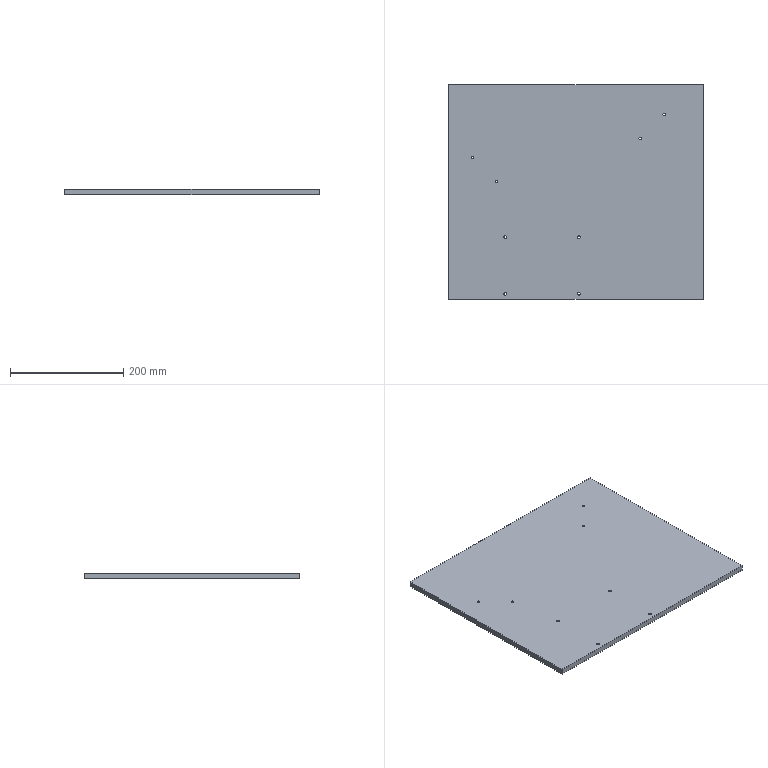Part | STEP file | 11-123211 | 1 solid | 22 faces | box 450 x 380 x 10 mm | volume 1708660 mm3 | cylinder 16 | plane 6 | commonest cylinder face diameters 4.2 x8 5 x8
STEP:
#1=CARTESIAN_POINT('',(153.683,136.933,10.));
#2=VERTEX_POINT('',#1);
#3=CARTESIAN_POINT('',(157.883,136.933,10.));
#4=VERTEX_POINT('',#3);
#5=CARTESIAN_POINT('',(155.783,136.933,10.));
#6=DIRECTION('',(0.,0.,1.));
#7=DIRECTION('',(1.,0.,0.));
#8=AXIS2_PLACEMENT_3D('',#5,#6,#7);
#9=CIRCLE('',#8,2.1);
#10=EDGE_CURVE('',#2,#4,#9,.T.);
#11=ORIENTED_EDGE('',*,*,#10,.T.);
#12=CARTESIAN_POINT('',(157.883,136.933,0.));
#13=VERTEX_POINT('',#12);
#14=CARTESIAN_POINT('',(157.883,136.933,0.));
#15=DIRECTION('',(0.,0.,-1.));
#16=VECTOR('',#15,1000.);
#17=LINE('',#14,#16);
#18=EDGE_CURVE('',#4,#13,#17,.T.);
#19=ORIENTED_EDGE('',*,*,#18,.T.);
#20=CARTESIAN_POINT('',(153.683,136.933,0.));
#21=VERTEX_POINT('',#20);
#22=CARTESIAN_POINT('',(155.783,136.933,0.));
#23=DIRECTION('',(0.,0.,-1.));
#24=DIRECTION('',(-1.,0.,0.));
#25=AXIS2_PLACEMENT_3D('',#22,#23,#24);
#26=CIRCLE('',#25,2.1);
#27=EDGE_CURVE('',#13,#21,#26,.T.);
#28=ORIENTED_EDGE('',*,*,#27,.T.);
#29=CARTESIAN_POINT('',(153.683,136.933,0.));
#30=DIRECTION('',(0.,0.,-1.));
#31=VECTOR('',#30,1000.);
#32=LINE('',#29,#31);
#33=EDGE_CURVE('',#2,#21,#32,.T.);
#34=ORIENTED_EDGE('',*,*,#33,.F.);
#35=EDGE_LOOP('',(#11,#19,#28,#34));
#36=FACE_OUTER_BOUND('',#35,.T.);
#37=CARTESIAN_POINT('',(155.783,136.933,0.));
#38=DIRECTION('',(0.,0.,-1.));
#39=DIRECTION('',(-1.,0.,0.));
#40=AXIS2_PLACEMENT_3D('',#37,#38,#39);
#41=CYLINDRICAL_SURFACE('',#40,2.1);
#42=ADVANCED_FACE('',(#36),#41,.F.);
#43=CARTESIAN_POINT('',(111.257,94.507,10.));
#44=VERTEX_POINT('',#43);
#45=CARTESIAN_POINT('',(115.457,94.507,10.));
#46=VERTEX_POINT('',#45);
#47=CARTESIAN_POINT('',(113.357,94.507,10.));
#48=DIRECTION('',(0.,0.,1.));
#49=DIRECTION('',(1.,0.,0.));
#50=AXIS2_PLACEMENT_3D('',#47,#48,#49);
#51=CIRCLE('',#50,2.1);
#52=EDGE_CURVE('',#44,#46,#51,.T.);
#53=ORIENTED_EDGE('',*,*,#52,.T.);
#54=CARTESIAN_POINT('',(115.457,94.507,0.));
#55=VERTEX_POINT('',#54);
#56=CARTESIAN_POINT('',(115.457,94.507,0.));
#57=DIRECTION('',(0.,0.,-1.));
#58=VECTOR('',#57,1000.);
#59=LINE('',#56,#58);
#60=EDGE_CURVE('',#46,#55,#59,.T.);
#61=ORIENTED_EDGE('',*,*,#60,.T.);
#62=CARTESIAN_POINT('',(111.257,94.507,0.));
#63=VERTEX_POINT('',#62);
#64=CARTESIAN_POINT('',(113.357,94.507,0.));
#65=DIRECTION('',(0.,0.,-1.));
#66=DIRECTION('',(-1.,0.,0.));
#67=AXIS2_PLACEMENT_3D('',#64,#65,#66);
#68=CIRCLE('',#67,2.1);
#69=EDGE_CURVE('',#55,#63,#68,.T.);
#70=ORIENTED_EDGE('',*,*,#69,.T.);
#71=CARTESIAN_POINT('',(111.257,94.507,0.));
#72=DIRECTION('',(0.,0.,-1.));
#73=VECTOR('',#72,1000.);
#74=LINE('',#71,#73);
#75=EDGE_CURVE('',#44,#63,#74,.T.);
#76=ORIENTED_EDGE('',*,*,#75,.F.);
#77=EDGE_LOOP('',(#53,#61,#70,#76));
#78=FACE_OUTER_BOUND('',#77,.T.);
#79=CARTESIAN_POINT('',(113.357,94.507,0.));
#80=DIRECTION('',(0.,0.,-1.));
#81=DIRECTION('',(-1.,0.,0.));
#82=AXIS2_PLACEMENT_3D('',#79,#80,#81);
#83=CYLINDRICAL_SURFACE('',#82,2.1);
#84=ADVANCED_FACE('',(#78),#83,.F.);
#85=CARTESIAN_POINT('',(-142.258,19.056,10.));
#86=VERTEX_POINT('',#85);
#87=CARTESIAN_POINT('',(-138.058,19.056,10.));
#88=VERTEX_POINT('',#87);
#89=CARTESIAN_POINT('',(-140.158,19.056,10.));
#90=DIRECTION('',(0.,0.,1.));
#91=DIRECTION('',(1.,0.,0.));
#92=AXIS2_PLACEMENT_3D('',#89,#90,#91);
#93=CIRCLE('',#92,2.1);
#94=EDGE_CURVE('',#86,#88,#93,.T.);
#95=ORIENTED_EDGE('',*,*,#94,.T.);
#96=CARTESIAN_POINT('',(-138.058,19.056,0.));
#97=VERTEX_POINT('',#96);
#98=CARTESIAN_POINT('',(-138.058,19.056,0.));
#99=DIRECTION('',(0.,0.,-1.));
#100=VECTOR('',#99,1000.);
#101=LINE('',#98,#100);
#102=EDGE_CURVE('',#88,#97,#101,.T.);
#103=ORIENTED_EDGE('',*,*,#102,.T.);
#104=CARTESIAN_POINT('',(-142.258,19.056,0.));
#105=VERTEX_POINT('',#104);
#106=CARTESIAN_POINT('',(-140.158,19.056,0.));
#107=DIRECTION('',(0.,0.,-1.));
#108=DIRECTION('',(-1.,0.,0.));
#109=AXIS2_PLACEMENT_3D('',#106,#107,#108);
#110=CIRCLE('',#109,2.1);
#111=EDGE_CURVE('',#97,#105,#110,.T.);
#112=ORIENTED_EDGE('',*,*,#111,.T.);
#113=CARTESIAN_POINT('',(-142.258,19.056,0.));
#114=DIRECTION('',(0.,0.,-1.));
#115=VECTOR('',#114,1000.);
#116=LINE('',#113,#115);
#117=EDGE_CURVE('',#86,#105,#116,.T.);
#118=ORIENTED_EDGE('',*,*,#117,.F.);
#119=EDGE_LOOP('',(#95,#103,#112,#118));
#120=FACE_OUTER_BOUND('',#119,.T.);
#121=CARTESIAN_POINT('',(-140.158,19.056,0.));
#122=DIRECTION('',(0.,0.,-1.));
#123=DIRECTION('',(-1.,0.,0.));
#124=AXIS2_PLACEMENT_3D('',#121,#122,#123);
#125=CYLINDRICAL_SURFACE('',#124,2.1);
#126=ADVANCED_FACE('',(#120),#125,.F.);
#127=CARTESIAN_POINT('',(-184.684,61.483,10.));
#128=VERTEX_POINT('',#127);
#129=CARTESIAN_POINT('',(-180.484,61.483,10.));
#130=VERTEX_POINT('',#129);
#131=CARTESIAN_POINT('',(-182.584,61.483,10.));
#132=DIRECTION('',(0.,0.,1.));
#133=DIRECTION('',(1.,0.,0.));
#134=AXIS2_PLACEMENT_3D('',#131,#132,#133);
#135=CIRCLE('',#134,2.1);
#136=EDGE_CURVE('',#128,#130,#135,.T.);
#137=ORIENTED_EDGE('',*,*,#136,.T.);
#138=CARTESIAN_POINT('',(-180.484,61.483,0.));
#139=VERTEX_POINT('',#138);
#140=CARTESIAN_POINT('',(-180.484,61.483,0.));
#141=DIRECTION('',(0.,0.,-1.));
#142=VECTOR('',#141,1000.);
#143=LINE('',#140,#142);
#144=EDGE_CURVE('',#130,#139,#143,.T.);
#145=ORIENTED_EDGE('',*,*,#144,.T.);
#146=CARTESIAN_POINT('',(-184.684,61.483,0.));
#147=VERTEX_POINT('',#146);
#148=CARTESIAN_POINT('',(-182.584,61.483,0.));
#149=DIRECTION('',(0.,0.,-1.));
#150=DIRECTION('',(-1.,0.,0.));
#151=AXIS2_PLACEMENT_3D('',#148,#149,#150);
#152=CIRCLE('',#151,2.1);
#153=EDGE_CURVE('',#139,#147,#152,.T.);
#154=ORIENTED_EDGE('',*,*,#153,.T.);
#155=CARTESIAN_POINT('',(-184.684,61.483,0.));
#156=DIRECTION('',(0.,0.,-1.));
#157=VECTOR('',#156,1000.);
#158=LINE('',#155,#157);
#159=EDGE_CURVE('',#128,#147,#158,.T.);
#160=ORIENTED_EDGE('',*,*,#159,.F.);
#161=EDGE_LOOP('',(#137,#145,#154,#160));
#162=FACE_OUTER_BOUND('',#161,.T.);
#163=CARTESIAN_POINT('',(-182.584,61.483,0.));
#164=DIRECTION('',(0.,0.,-1.));
#165=DIRECTION('',(-1.,0.,0.));
#166=AXIS2_PLACEMENT_3D('',#163,#164,#165);
#167=CYLINDRICAL_SURFACE('',#166,2.1);
#168=ADVANCED_FACE('',(#162),#167,.F.);
#169=CARTESIAN_POINT('',(-127.5,-80.,10.));
#170=VERTEX_POINT('',#169);
#171=CARTESIAN_POINT('',(-122.5,-80.,10.));
#172=VERTEX_POINT('',#171);
#173=CARTESIAN_POINT('',(-125.,-80.,10.));
#174=DIRECTION('',(0.,0.,1.));
#175=DIRECTION('',(1.,0.,0.));
#176=AXIS2_PLACEMENT_3D('',#173,#174,#175);
#177=CIRCLE('',#176,2.5);
#178=EDGE_CURVE('',#170,#172,#177,.T.);
#179=ORIENTED_EDGE('',*,*,#178,.T.);
#180=CARTESIAN_POINT('',(-122.5,-80.,0.));
#181=VERTEX_POINT('',#180);
#182=CARTESIAN_POINT('',(-122.5,-80.,0.));
#183=DIRECTION('',(0.,0.,-1.));
#184=VECTOR('',#183,1000.);
#185=LINE('',#182,#184);
#186=EDGE_CURVE('',#172,#181,#185,.T.);
#187=ORIENTED_EDGE('',*,*,#186,.T.);
#188=CARTESIAN_POINT('',(-127.5,-80.,0.));
#189=VERTEX_POINT('',#188);
#190=CARTESIAN_POINT('',(-125.,-80.,0.));
#191=DIRECTION('',(0.,0.,-1.));
#192=DIRECTION('',(-1.,0.,0.));
#193=AXIS2_PLACEMENT_3D('',#190,#191,#192);
#194=CIRCLE('',#193,2.5);
#195=EDGE_CURVE('',#181,#189,#194,.T.);
#196=ORIENTED_EDGE('',*,*,#195,.T.);
#197=CARTESIAN_POINT('',(-127.5,-80.,0.));
#198=DIRECTION('',(0.,0.,-1.));
#199=VECTOR('',#198,1000.);
#200=LINE('',#197,#199);
#201=EDGE_CURVE('',#170,#189,#200,.T.);
#202=ORIENTED_EDGE('',*,*,#201,.F.);
#203=EDGE_LOOP('',(#179,#187,#196,#202));
#204=FACE_OUTER_BOUND('',#203,.T.);
#205=CARTESIAN_POINT('',(-125.,-80.,0.));
#206=DIRECTION('',(0.,0.,-1.));
#207=DIRECTION('',(-1.,0.,0.));
#208=AXIS2_PLACEMENT_3D('',#205,#206,#207);
#209=CYLINDRICAL_SURFACE('',#208,2.5);
#210=ADVANCED_FACE('',(#204),#209,.F.);
#211=CARTESIAN_POINT('',(-127.5,-180.,10.));
#212=VERTEX_POINT('',#211);
#213=CARTESIAN_POINT('',(-122.5,-180.,10.));
#214=VERTEX_POINT('',#213);
#215=CARTESIAN_POINT('',(-125.,-180.,10.));
#216=DIRECTION('',(0.,0.,1.));
#217=DIRECTION('',(1.,0.,0.));
#218=AXIS2_PLACEMENT_3D('',#215,#216,#217);
#219=CIRCLE('',#218,2.5);
#220=EDGE_CURVE('',#212,#214,#219,.T.);
#221=ORIENTED_EDGE('',*,*,#220,.T.);
#222=CARTESIAN_POINT('',(-122.5,-180.,0.));
#223=VERTEX_POINT('',#222);
#224=CARTESIAN_POINT('',(-122.5,-180.,0.));
#225=DIRECTION('',(0.,0.,-1.));
#226=VECTOR('',#225,1000.);
#227=LINE('',#224,#226);
#228=EDGE_CURVE('',#214,#223,#227,.T.);
#229=ORIENTED_EDGE('',*,*,#228,.T.);
#230=CARTESIAN_POINT('',(-127.5,-180.,0.));
#231=VERTEX_POINT('',#230);
#232=CARTESIAN_POINT('',(-125.,-180.,0.));
#233=DIRECTION('',(0.,0.,-1.));
#234=DIRECTION('',(-1.,0.,0.));
#235=AXIS2_PLACEMENT_3D('',#232,#233,#234);
#236=CIRCLE('',#235,2.5);
#237=EDGE_CURVE('',#223,#231,#236,.T.);
#238=ORIENTED_EDGE('',*,*,#237,.T.);
#239=CARTESIAN_POINT('',(-127.5,-180.,0.));
#240=DIRECTION('',(0.,0.,-1.));
#241=VECTOR('',#240,1000.);
#242=LINE('',#239,#241);
#243=EDGE_CURVE('',#212,#231,#242,.T.);
#244=ORIENTED_EDGE('',*,*,#243,.F.);
#245=EDGE_LOOP('',(#221,#229,#238,#244));
#246=FACE_OUTER_BOUND('',#245,.T.);
#247=CARTESIAN_POINT('',(-125.,-180.,0.));
#248=DIRECTION('',(0.,0.,-1.));
#249=DIRECTION('',(-1.,0.,0.));
#250=AXIS2_PLACEMENT_3D('',#247,#248,#249);
#251=CYLINDRICAL_SURFACE('',#250,2.5);
#252=ADVANCED_FACE('',(#246),#251,.F.);
#253=CARTESIAN_POINT('',(2.5,-180.,10.));
#254=VERTEX_POINT('',#253);
#255=CARTESIAN_POINT('',(7.5,-180.,10.));
#256=VERTEX_POINT('',#255);
#257=CARTESIAN_POINT('',(5.,-180.,10.));
#258=DIRECTION('',(0.,0.,1.));
#259=DIRECTION('',(1.,0.,0.));
#260=AXIS2_PLACEMENT_3D('',#257,#258,#259);
#261=CIRCLE('',#260,2.5);
#262=EDGE_CURVE('',#254,#256,#261,.T.);
#263=ORIENTED_EDGE('',*,*,#262,.T.);
#264=CARTESIAN_POINT('',(7.5,-180.,0.));
#265=VERTEX_POINT('',#264);
#266=CARTESIAN_POINT('',(7.5,-180.,0.));
#267=DIRECTION('',(0.,0.,-1.));
#268=VECTOR('',#267,1000.);
#269=LINE('',#266,#268);
#270=EDGE_CURVE('',#256,#265,#269,.T.);
#271=ORIENTED_EDGE('',*,*,#270,.T.);
#272=CARTESIAN_POINT('',(2.5,-180.,0.));
#273=VERTEX_POINT('',#272);
#274=CARTESIAN_POINT('',(5.,-180.,0.));
#275=DIRECTION('',(0.,0.,-1.));
#276=DIRECTION('',(-1.,0.,0.));
#277=AXIS2_PLACEMENT_3D('',#274,#275,#276);
#278=CIRCLE('',#277,2.5);
#279=EDGE_CURVE('',#265,#273,#278,.T.);
#280=ORIENTED_EDGE('',*,*,#279,.T.);
#281=CARTESIAN_POINT('',(2.5,-180.,0.));
#282=DIRECTION('',(0.,0.,-1.));
#283=VECTOR('',#282,1000.);
#284=LINE('',#281,#283);
#285=EDGE_CURVE('',#254,#273,#284,.T.);
#286=ORIENTED_EDGE('',*,*,#285,.F.);
#287=EDGE_LOOP('',(#263,#271,#280,#286));
#288=FACE_OUTER_BOUND('',#287,.T.);
#289=CARTESIAN_POINT('',(5.,-180.,0.));
#290=DIRECTION('',(0.,0.,-1.));
#291=DIRECTION('',(-1.,0.,0.));
#292=AXIS2_PLACEMENT_3D('',#289,#290,#291);
#293=CYLINDRICAL_SURFACE('',#292,2.5);
#294=ADVANCED_FACE('',(#288),#293,.F.);
#295=CARTESIAN_POINT('',(2.5,-80.,10.));
#296=VERTEX_POINT('',#295);
#297=CARTESIAN_POINT('',(7.5,-80.,10.));
#298=VERTEX_POINT('',#297);
#299=CARTESIAN_POINT('',(5.,-80.,10.));
#300=DIRECTION('',(0.,0.,1.));
#301=DIRECTION('',(1.,0.,0.));
#302=AXIS2_PLACEMENT_3D('',#299,#300,#301);
#303=CIRCLE('',#302,2.5);
#304=EDGE_CURVE('',#296,#298,#303,.T.);
#305=ORIENTED_EDGE('',*,*,#304,.T.);
#306=CARTESIAN_POINT('',(7.5,-80.,0.));
#307=VERTEX_POINT('',#306);
#308=CARTESIAN_POINT('',(7.5,-80.,0.));
#309=DIRECTION('',(0.,0.,-1.));
#310=VECTOR('',#309,1000.);
#311=LINE('',#308,#310);
#312=EDGE_CURVE('',#298,#307,#311,.T.);
#313=ORIENTED_EDGE('',*,*,#312,.T.);
#314=CARTESIAN_POINT('',(2.5,-80.,0.));
#315=VERTEX_POINT('',#314);
#316=CARTESIAN_POINT('',(5.,-80.,0.));
#317=DIRECTION('',(0.,0.,-1.));
#318=DIRECTION('',(-1.,0.,0.));
#319=AXIS2_PLACEMENT_3D('',#316,#317,#318);
#320=CIRCLE('',#319,2.5);
#321=EDGE_CURVE('',#307,#315,#320,.T.);
#322=ORIENTED_EDGE('',*,*,#321,.T.);
#323=CARTESIAN_POINT('',(2.5,-80.,0.));
#324=DIRECTION('',(0.,0.,-1.));
#325=VECTOR('',#324,1000.);
#326=LINE('',#323,#325);
#327=EDGE_CURVE('',#296,#315,#326,.T.);
#328=ORIENTED_EDGE('',*,*,#327,.F.);
#329=EDGE_LOOP('',(#305,#313,#322,#328));
#330=FACE_OUTER_BOUND('',#329,.T.);
#331=CARTESIAN_POINT('',(5.,-80.,0.));
#332=DIRECTION('',(0.,0.,-1.));
#333=DIRECTION('',(-1.,0.,0.));
#334=AXIS2_PLACEMENT_3D('',#331,#332,#333);
#335=CYLINDRICAL_SURFACE('',#334,2.5);
#336=ADVANCED_FACE('',(#330),#335,.F.);
#337=CARTESIAN_POINT('',(225.,-190.,0.));
#338=VERTEX_POINT('',#337);
#339=CARTESIAN_POINT('',(225.,190.,0.));
#340=VERTEX_POINT('',#339);
#341=CARTESIAN_POINT('',(225.,190.,0.));
#342=DIRECTION('',(0.,1.,0.));
#343=VECTOR('',#342,1000.);
#344=LINE('',#341,#343);
#345=EDGE_CURVE('',#338,#340,#344,.T.);
#346=ORIENTED_EDGE('',*,*,#345,.T.);
#347=CARTESIAN_POINT('',(225.,190.,10.));
#348=VERTEX_POINT('',#347);
#349=CARTESIAN_POINT('',(225.,190.,10.));
#350=DIRECTION('',(0.,0.,-1.));
#351=VECTOR('',#350,1000.);
#352=LINE('',#349,#351);
#353=EDGE_CURVE('',#348,#340,#352,.T.);
#354=ORIENTED_EDGE('',*,*,#353,.F.);
#355=CARTESIAN_POINT('',(225.,-190.,10.));
#356=VERTEX_POINT('',#355);
#357=CARTESIAN_POINT('',(225.,190.,10.));
#358=DIRECTION('',(0.,1.,0.));
#359=VECTOR('',#358,1000.);
#360=LINE('',#357,#359);
#361=EDGE_CURVE('',#356,#348,#360,.T.);
#362=ORIENTED_EDGE('',*,*,#361,.F.);
#363=CARTESIAN_POINT('',(225.,-190.,10.));
#364=DIRECTION('',(0.,0.,-1.));
#365=VECTOR('',#364,1000.);
#366=LINE('',#363,#365);
#367=EDGE_CURVE('',#356,#338,#366,.T.);
#368=ORIENTED_EDGE('',*,*,#367,.T.);
#369=EDGE_LOOP('',(#346,#354,#362,#368));
#370=FACE_OUTER_BOUND('',#369,.T.);
#371=CARTESIAN_POINT('',(225.,190.,10.));
#372=DIRECTION('',(-1.,0.,0.));
#373=DIRECTION('',(0.,-1.,0.));
#374=AXIS2_PLACEMENT_3D('',#371,#372,#373);
#375=PLANE('',#374);
#376=ADVANCED_FACE('',(#370),#375,.F.);
#377=CARTESIAN_POINT('',(-225.,190.,0.));
#378=VERTEX_POINT('',#377);
#379=CARTESIAN_POINT('',(-225.,190.,0.));
#380=DIRECTION('',(-1.,0.,0.));
#381=VECTOR('',#380,1000.);
#382=LINE('',#379,#381);
#383=EDGE_CURVE('',#340,#378,#382,.T.);
#384=ORIENTED_EDGE('',*,*,#383,.T.);
#385=CARTESIAN_POINT('',(-225.,190.,10.));
#386=VERTEX_POINT('',#385);
#387=CARTESIAN_POINT('',(-225.,190.,10.));
#388=DIRECTION('',(0.,0.,-1.));
#389=VECTOR('',#388,1000.);
#390=LINE('',#387,#389);
#391=EDGE_CURVE('',#386,#378,#390,.T.);
#392=ORIENTED_EDGE('',*,*,#391,.F.);
#393=CARTESIAN_POINT('',(-225.,190.,10.));
#394=DIRECTION('',(-1.,0.,0.));
#395=VECTOR('',#394,1000.);
#396=LINE('',#393,#395);
#397=EDGE_CURVE('',#348,#386,#396,.T.);
#398=ORIENTED_EDGE('',*,*,#397,.F.);
#399=ORIENTED_EDGE('',*,*,#353,.T.);
#400=EDGE_LOOP('',(#384,#392,#398,#399));
#401=FACE_OUTER_BOUND('',#400,.T.);
#402=CARTESIAN_POINT('',(-225.,190.,10.));
#403=DIRECTION('',(0.,-1.,0.));
#404=DIRECTION('',(0.,0.,-1.));
#405=AXIS2_PLACEMENT_3D('',#402,#403,#404);
#406=PLANE('',#405);
#407=ADVANCED_FACE('',(#401),#406,.F.);
#408=CARTESIAN_POINT('',(-225.,-190.,0.));
#409=VERTEX_POINT('',#408);
#410=CARTESIAN_POINT('',(-225.,190.,0.));
#411=DIRECTION('',(0.,-1.,0.));
#412=VECTOR('',#411,1000.);
#413=LINE('',#410,#412);
#414=EDGE_CURVE('',#378,#409,#413,.T.);
#415=ORIENTED_EDGE('',*,*,#414,.T.);
#416=CARTESIAN_POINT('',(-225.,-190.,10.));
#417=VERTEX_POINT('',#416);
#418=CARTESIAN_POINT('',(-225.,-190.,10.));
#419=DIRECTION('',(0.,0.,-1.));
#420=VECTOR('',#419,1000.);
#421=LINE('',#418,#420);
#422=EDGE_CURVE('',#417,#409,#421,.T.);
#423=ORIENTED_EDGE('',*,*,#422,.F.);
#424=CARTESIAN_POINT('',(-225.,190.,10.));
#425=DIRECTION('',(0.,-1.,0.));
#426=VECTOR('',#425,1000.);
#427=LINE('',#424,#426);
#428=EDGE_CURVE('',#386,#417,#427,.T.);
#429=ORIENTED_EDGE('',*,*,#428,.F.);
#430=ORIENTED_EDGE('',*,*,#391,.T.);
#431=EDGE_LOOP('',(#415,#423,#429,#430));
#432=FACE_OUTER_BOUND('',#431,.T.);
#433=CARTESIAN_POINT('',(-225.,190.,10.));
#434=DIRECTION('',(1.,0.,0.));
#435=DIRECTION('',(0.,1.,0.));
#436=AXIS2_PLACEMENT_3D('',#433,#434,#435);
#437=PLANE('',#436);
#438=ADVANCED_FACE('',(#432),#437,.F.);
#439=CARTESIAN_POINT('',(-225.,-190.,0.));
#440=DIRECTION('',(1.,0.,0.));
#441=VECTOR('',#440,1000.);
#442=LINE('',#439,#441);
#443=EDGE_CURVE('',#409,#338,#442,.T.);
#444=ORIENTED_EDGE('',*,*,#443,.T.);
#445=ORIENTED_EDGE('',*,*,#367,.F.);
#446=CARTESIAN_POINT('',(-225.,-190.,10.));
#447=DIRECTION('',(1.,0.,0.));
#448=VECTOR('',#447,1000.);
#449=LINE('',#446,#448);
#450=EDGE_CURVE('',#417,#356,#449,.T.);
#451=ORIENTED_EDGE('',*,*,#450,.F.);
#452=ORIENTED_EDGE('',*,*,#422,.T.);
#453=EDGE_LOOP('',(#444,#445,#451,#452));
#454=FACE_OUTER_BOUND('',#453,.T.);
#455=CARTESIAN_POINT('',(-225.,-190.,10.));
#456=DIRECTION('',(0.,1.,0.));
#457=DIRECTION('',(0.,0.,1.));
#458=AXIS2_PLACEMENT_3D('',#455,#456,#457);
#459=PLANE('',#458);
#460=ADVANCED_FACE('',(#454),#459,.F.);
#461=ORIENTED_EDGE('',*,*,#10,.F.);
#462=CARTESIAN_POINT('',(155.783,136.933,10.));
#463=DIRECTION('',(0.,0.,1.));
#464=DIRECTION('',(1.,0.,0.));
#465=AXIS2_PLACEMENT_3D('',#462,#463,#464);
#466=CIRCLE('',#465,2.1);
#467=EDGE_CURVE('',#4,#2,#466,.T.);
#468=ORIENTED_EDGE('',*,*,#467,.F.);
#469=EDGE_LOOP('',(#461,#468));
#470=FACE_BOUND('',#469,.T.);
#471=ORIENTED_EDGE('',*,*,#52,.F.);
#472=CARTESIAN_POINT('',(113.357,94.507,10.));
#473=DIRECTION('',(0.,0.,1.));
#474=DIRECTION('',(1.,0.,0.));
#475=AXIS2_PLACEMENT_3D('',#472,#473,#474);
#476=CIRCLE('',#475,2.1);
#477=EDGE_CURVE('',#46,#44,#476,.T.);
#478=ORIENTED_EDGE('',*,*,#477,.F.);
#479=EDGE_LOOP('',(#471,#478));
#480=FACE_BOUND('',#479,.T.);
#481=ORIENTED_EDGE('',*,*,#94,.F.);
#482=CARTESIAN_POINT('',(-140.158,19.056,10.));
#483=DIRECTION('',(0.,0.,1.));
#484=DIRECTION('',(1.,0.,0.));
#485=AXIS2_PLACEMENT_3D('',#482,#483,#484);
#486=CIRCLE('',#485,2.1);
#487=EDGE_CURVE('',#88,#86,#486,.T.);
#488=ORIENTED_EDGE('',*,*,#487,.F.);
#489=EDGE_LOOP('',(#481,#488));
#490=FACE_BOUND('',#489,.T.);
#491=ORIENTED_EDGE('',*,*,#136,.F.);
#492=CARTESIAN_POINT('',(-182.584,61.483,10.));
#493=DIRECTION('',(0.,0.,1.));
#494=DIRECTION('',(1.,0.,0.));
#495=AXIS2_PLACEMENT_3D('',#492,#493,#494);
#496=CIRCLE('',#495,2.1);
#497=EDGE_CURVE('',#130,#128,#496,.T.);
#498=ORIENTED_EDGE('',*,*,#497,.F.);
#499=EDGE_LOOP('',(#491,#498));
#500=FACE_BOUND('',#499,.T.);
#501=ORIENTED_EDGE('',*,*,#178,.F.);
#502=CARTESIAN_POINT('',(-125.,-80.,10.));
#503=DIRECTION('',(0.,0.,1.));
#504=DIRECTION('',(1.,0.,0.));
#505=AXIS2_PLACEMENT_3D('',#502,#503,#504);
#506=CIRCLE('',#505,2.5);
#507=EDGE_CURVE('',#172,#170,#506,.T.);
#508=ORIENTED_EDGE('',*,*,#507,.F.);
#509=EDGE_LOOP('',(#501,#508));
#510=FACE_BOUND('',#509,.T.);
#511=ORIENTED_EDGE('',*,*,#220,.F.);
#512=CARTESIAN_POINT('',(-125.,-180.,10.));
#513=DIRECTION('',(0.,0.,1.));
#514=DIRECTION('',(1.,0.,0.));
#515=AXIS2_PLACEMENT_3D('',#512,#513,#514);
#516=CIRCLE('',#515,2.5);
#517=EDGE_CURVE('',#214,#212,#516,.T.);
#518=ORIENTED_EDGE('',*,*,#517,.F.);
#519=EDGE_LOOP('',(#511,#518));
#520=FACE_BOUND('',#519,.T.);
#521=ORIENTED_EDGE('',*,*,#262,.F.);
#522=CARTESIAN_POINT('',(5.,-180.,10.));
#523=DIRECTION('',(0.,0.,1.));
#524=DIRECTION('',(1.,0.,0.));
#525=AXIS2_PLACEMENT_3D('',#522,#523,#524);
#526=CIRCLE('',#525,2.5);
#527=EDGE_CURVE('',#256,#254,#526,.T.);
#528=ORIENTED_EDGE('',*,*,#527,.F.);
#529=EDGE_LOOP('',(#521,#528));
#530=FACE_BOUND('',#529,.T.);
#531=ORIENTED_EDGE('',*,*,#304,.F.);
#532=CARTESIAN_POINT('',(5.,-80.,10.));
#533=DIRECTION('',(0.,0.,1.));
#534=DIRECTION('',(1.,0.,0.));
#535=AXIS2_PLACEMENT_3D('',#532,#533,#534);
#536=CIRCLE('',#535,2.5);
#537=EDGE_CURVE('',#298,#296,#536,.T.);
#538=ORIENTED_EDGE('',*,*,#537,.F.);
#539=EDGE_LOOP('',(#531,#538));
#540=FACE_BOUND('',#539,.T.);
#541=ORIENTED_EDGE('',*,*,#361,.T.);
#542=ORIENTED_EDGE('',*,*,#397,.T.);
#543=ORIENTED_EDGE('',*,*,#428,.T.);
#544=ORIENTED_EDGE('',*,*,#450,.T.);
#545=EDGE_LOOP('',(#541,#542,#543,#544));
#546=FACE_OUTER_BOUND('',#545,.T.);
#547=CARTESIAN_POINT('',(0.,0.,10.));
#548=DIRECTION('',(0.,0.,1.));
#549=DIRECTION('',(1.,0.,0.));
#550=AXIS2_PLACEMENT_3D('',#547,#548,#549);
#551=PLANE('',#550);
#552=ADVANCED_FACE('',(#470,#480,#490,#500,#510,#520,#530,#540,#546),#551,.T.);
#553=CARTESIAN_POINT('',(155.783,136.933,0.));
#554=DIRECTION('',(0.,0.,-1.));
#555=DIRECTION('',(-1.,0.,0.));
#556=AXIS2_PLACEMENT_3D('',#553,#554,#555);
#557=CIRCLE('',#556,2.1);
#558=EDGE_CURVE('',#21,#13,#557,.T.);
#559=ORIENTED_EDGE('',*,*,#558,.F.);
#560=ORIENTED_EDGE('',*,*,#27,.F.);
#561=EDGE_LOOP('',(#559,#560));
#562=FACE_BOUND('',#561,.T.);
#563=CARTESIAN_POINT('',(113.357,94.507,0.));
#564=DIRECTION('',(0.,0.,-1.));
#565=DIRECTION('',(-1.,0.,0.));
#566=AXIS2_PLACEMENT_3D('',#563,#564,#565);
#567=CIRCLE('',#566,2.1);
#568=EDGE_CURVE('',#63,#55,#567,.T.);
#569=ORIENTED_EDGE('',*,*,#568,.F.);
#570=ORIENTED_EDGE('',*,*,#69,.F.);
#571=EDGE_LOOP('',(#569,#570));
#572=FACE_BOUND('',#571,.T.);
#573=CARTESIAN_POINT('',(-140.158,19.056,0.));
#574=DIRECTION('',(0.,0.,-1.));
#575=DIRECTION('',(-1.,0.,0.));
#576=AXIS2_PLACEMENT_3D('',#573,#574,#575);
#577=CIRCLE('',#576,2.1);
#578=EDGE_CURVE('',#105,#97,#577,.T.);
#579=ORIENTED_EDGE('',*,*,#578,.F.);
#580=ORIENTED_EDGE('',*,*,#111,.F.);
#581=EDGE_LOOP('',(#579,#580));
#582=FACE_BOUND('',#581,.T.);
#583=CARTESIAN_POINT('',(-182.584,61.483,0.));
#584=DIRECTION('',(0.,0.,-1.));
#585=DIRECTION('',(-1.,0.,0.));
#586=AXIS2_PLACEMENT_3D('',#583,#584,#585);
#587=CIRCLE('',#586,2.1);
#588=EDGE_CURVE('',#147,#139,#587,.T.);
#589=ORIENTED_EDGE('',*,*,#588,.F.);
#590=ORIENTED_EDGE('',*,*,#153,.F.);
#591=EDGE_LOOP('',(#589,#590));
#592=FACE_BOUND('',#591,.T.);
#593=CARTESIAN_POINT('',(-125.,-80.,0.));
#594=DIRECTION('',(0.,0.,-1.));
#595=DIRECTION('',(-1.,0.,0.));
#596=AXIS2_PLACEMENT_3D('',#593,#594,#595);
#597=CIRCLE('',#596,2.5);
#598=EDGE_CURVE('',#189,#181,#597,.T.);
#599=ORIENTED_EDGE('',*,*,#598,.F.);
#600=ORIENTED_EDGE('',*,*,#195,.F.);
#601=EDGE_LOOP('',(#599,#600));
#602=FACE_BOUND('',#601,.T.);
#603=CARTESIAN_POINT('',(-125.,-180.,0.));
#604=DIRECTION('',(0.,0.,-1.));
#605=DIRECTION('',(-1.,0.,0.));
#606=AXIS2_PLACEMENT_3D('',#603,#604,#605);
#607=CIRCLE('',#606,2.5);
#608=EDGE_CURVE('',#231,#223,#607,.T.);
#609=ORIENTED_EDGE('',*,*,#608,.F.);
#610=ORIENTED_EDGE('',*,*,#237,.F.);
#611=EDGE_LOOP('',(#609,#610));
#612=FACE_BOUND('',#611,.T.);
#613=CARTESIAN_POINT('',(5.,-180.,0.));
#614=DIRECTION('',(0.,0.,-1.));
#615=DIRECTION('',(-1.,0.,0.));
#616=AXIS2_PLACEMENT_3D('',#613,#614,#615);
#617=CIRCLE('',#616,2.5);
#618=EDGE_CURVE('',#273,#265,#617,.T.);
#619=ORIENTED_EDGE('',*,*,#618,.F.);
#620=ORIENTED_EDGE('',*,*,#279,.F.);
#621=EDGE_LOOP('',(#619,#620));
#622=FACE_BOUND('',#621,.T.);
#623=CARTESIAN_POINT('',(5.,-80.,0.));
#624=DIRECTION('',(0.,0.,-1.));
#625=DIRECTION('',(-1.,0.,0.));
#626=AXIS2_PLACEMENT_3D('',#623,#624,#625);
#627=CIRCLE('',#626,2.5);
#628=EDGE_CURVE('',#315,#307,#627,.T.);
#629=ORIENTED_EDGE('',*,*,#628,.F.);
#630=ORIENTED_EDGE('',*,*,#321,.F.);
#631=EDGE_LOOP('',(#629,#630));
#632=FACE_BOUND('',#631,.T.);
#633=ORIENTED_EDGE('',*,*,#345,.F.);
#634=ORIENTED_EDGE('',*,*,#443,.F.);
#635=ORIENTED_EDGE('',*,*,#414,.F.);
#636=ORIENTED_EDGE('',*,*,#383,.F.);
#637=EDGE_LOOP('',(#633,#634,#635,#636));
#638=FACE_OUTER_BOUND('',#637,.T.);
#639=CARTESIAN_POINT('',(0.,0.,0.));
#640=DIRECTION('',(0.,0.,1.));
#641=DIRECTION('',(1.,0.,0.));
#642=AXIS2_PLACEMENT_3D('',#639,#640,#641);
#643=PLANE('',#642);
#644=ADVANCED_FACE('',(#562,#572,#582,#592,#602,#612,#622,#632,#638),#643,.F.);
#645=ORIENTED_EDGE('',*,*,#312,.F.);
#646=ORIENTED_EDGE('',*,*,#537,.T.);
#647=ORIENTED_EDGE('',*,*,#327,.T.);
#648=ORIENTED_EDGE('',*,*,#628,.T.);
#649=EDGE_LOOP('',(#645,#646,#647,#648));
#650=FACE_OUTER_BOUND('',#649,.T.);
#651=CARTESIAN_POINT('',(5.,-80.,0.));
#652=DIRECTION('',(0.,0.,-1.));
#653=DIRECTION('',(-1.,0.,0.));
#654=AXIS2_PLACEMENT_3D('',#651,#652,#653);
#655=CYLINDRICAL_SURFACE('',#654,2.5);
#656=ADVANCED_FACE('',(#650),#655,.F.);
#657=ORIENTED_EDGE('',*,*,#270,.F.);
#658=ORIENTED_EDGE('',*,*,#527,.T.);
#659=ORIENTED_EDGE('',*,*,#285,.T.);
#660=ORIENTED_EDGE('',*,*,#618,.T.);
#661=EDGE_LOOP('',(#657,#658,#659,#660));
#662=FACE_OUTER_BOUND('',#661,.T.);
#663=CARTESIAN_POINT('',(5.,-180.,0.));
#664=DIRECTION('',(0.,0.,-1.));
#665=DIRECTION('',(-1.,0.,0.));
#666=AXIS2_PLACEMENT_3D('',#663,#664,#665);
#667=CYLINDRICAL_SURFACE('',#666,2.5);
#668=ADVANCED_FACE('',(#662),#667,.F.);
#669=ORIENTED_EDGE('',*,*,#228,.F.);
#670=ORIENTED_EDGE('',*,*,#517,.T.);
#671=ORIENTED_EDGE('',*,*,#243,.T.);
#672=ORIENTED_EDGE('',*,*,#608,.T.);
#673=EDGE_LOOP('',(#669,#670,#671,#672));
#674=FACE_OUTER_BOUND('',#673,.T.);
#675=CARTESIAN_POINT('',(-125.,-180.,0.));
#676=DIRECTION('',(0.,0.,-1.));
#677=DIRECTION('',(-1.,0.,0.));
#678=AXIS2_PLACEMENT_3D('',#675,#676,#677);
#679=CYLINDRICAL_SURFACE('',#678,2.5);
#680=ADVANCED_FACE('',(#674),#679,.F.);
#681=ORIENTED_EDGE('',*,*,#186,.F.);
#682=ORIENTED_EDGE('',*,*,#507,.T.);
#683=ORIENTED_EDGE('',*,*,#201,.T.);
#684=ORIENTED_EDGE('',*,*,#598,.T.);
#685=EDGE_LOOP('',(#681,#682,#683,#684));
#686=FACE_OUTER_BOUND('',#685,.T.);
#687=CARTESIAN_POINT('',(-125.,-80.,0.));
#688=DIRECTION('',(0.,0.,-1.));
#689=DIRECTION('',(-1.,0.,0.));
#690=AXIS2_PLACEMENT_3D('',#687,#688,#689);
#691=CYLINDRICAL_SURFACE('',#690,2.5);
#692=ADVANCED_FACE('',(#686),#691,.F.);
#693=ORIENTED_EDGE('',*,*,#144,.F.);
#694=ORIENTED_EDGE('',*,*,#497,.T.);
#695=ORIENTED_EDGE('',*,*,#159,.T.);
#696=ORIENTED_EDGE('',*,*,#588,.T.);
#697=EDGE_LOOP('',(#693,#694,#695,#696));
#698=FACE_OUTER_BOUND('',#697,.T.);
#699=CARTESIAN_POINT('',(-182.584,61.483,0.));
#700=DIRECTION('',(0.,0.,-1.));
#701=DIRECTION('',(-1.,0.,0.));
#702=AXIS2_PLACEMENT_3D('',#699,#700,#701);
#703=CYLINDRICAL_SURFACE('',#702,2.1);
#704=ADVANCED_FACE('',(#698),#703,.F.);
#705=ORIENTED_EDGE('',*,*,#102,.F.);
#706=ORIENTED_EDGE('',*,*,#487,.T.);
#707=ORIENTED_EDGE('',*,*,#117,.T.);
#708=ORIENTED_EDGE('',*,*,#578,.T.);
#709=EDGE_LOOP('',(#705,#706,#707,#708));
#710=FACE_OUTER_BOUND('',#709,.T.);
#711=CARTESIAN_POINT('',(-140.158,19.056,0.));
#712=DIRECTION('',(0.,0.,-1.));
#713=DIRECTION('',(-1.,0.,0.));
#714=AXIS2_PLACEMENT_3D('',#711,#712,#713);
#715=CYLINDRICAL_SURFACE('',#714,2.1);
#716=ADVANCED_FACE('',(#710),#715,.F.);
#717=ORIENTED_EDGE('',*,*,#60,.F.);
#718=ORIENTED_EDGE('',*,*,#477,.T.);
#719=ORIENTED_EDGE('',*,*,#75,.T.);
#720=ORIENTED_EDGE('',*,*,#568,.T.);
#721=EDGE_LOOP('',(#717,#718,#719,#720));
#722=FACE_OUTER_BOUND('',#721,.T.);
#723=CARTESIAN_POINT('',(113.357,94.507,0.));
#724=DIRECTION('',(0.,0.,-1.));
#725=DIRECTION('',(-1.,0.,0.));
#726=AXIS2_PLACEMENT_3D('',#723,#724,#725);
#727=CYLINDRICAL_SURFACE('',#726,2.1);
#728=ADVANCED_FACE('',(#722),#727,.F.);
#729=ORIENTED_EDGE('',*,*,#18,.F.);
#730=ORIENTED_EDGE('',*,*,#467,.T.);
#731=ORIENTED_EDGE('',*,*,#33,.T.);
#732=ORIENTED_EDGE('',*,*,#558,.T.);
#733=EDGE_LOOP('',(#729,#730,#731,#732));
#734=FACE_OUTER_BOUND('',#733,.T.);
#735=CARTESIAN_POINT('',(155.783,136.933,0.));
#736=DIRECTION('',(0.,0.,-1.));
#737=DIRECTION('',(-1.,0.,0.));
#738=AXIS2_PLACEMENT_3D('',#735,#736,#737);
#739=CYLINDRICAL_SURFACE('',#738,2.1);
#740=ADVANCED_FACE('',(#734),#739,.F.);
#741=CLOSED_SHELL('',(#42,#84,#126,#168,#210,#252,#294,#336,#376,#407,#438,#460,#552,#644,#656,#668,#680,#692,#704,#716,#728,#740));
#742=MANIFOLD_SOLID_BREP('',#741);
#743=CARTESIAN_POINT('',(0.,0.,0.));
#744=DIRECTION('',(0.,0.,1.));
#745=DIRECTION('',(1.,0.,0.));
#746=AXIS2_PLACEMENT_3D('',#743,#744,#745);
#747=(LENGTH_UNIT()NAMED_UNIT(*)SI_UNIT(.MILLI.,.METRE.));
#748=UNCERTAINTY_MEASURE_WITH_UNIT(LENGTH_MEASURE(0.00001),#747,'','');
#749=(NAMED_UNIT(*)PLANE_ANGLE_UNIT()SI_UNIT($,.RADIAN.));
#750=(NAMED_UNIT(*)SI_UNIT($,.STERADIAN.)SOLID_ANGLE_UNIT());
#751=(GEOMETRIC_REPRESENTATION_CONTEXT(3)GLOBAL_UNCERTAINTY_ASSIGNED_CONTEXT((#748))GLOBAL_UNIT_ASSIGNED_CONTEXT((#747,#749,#750))REPRESENTATION_CONTEXT('',''));
#752=ADVANCED_BREP_SHAPE_REPRESENTATION('',(#742,#746),#751);